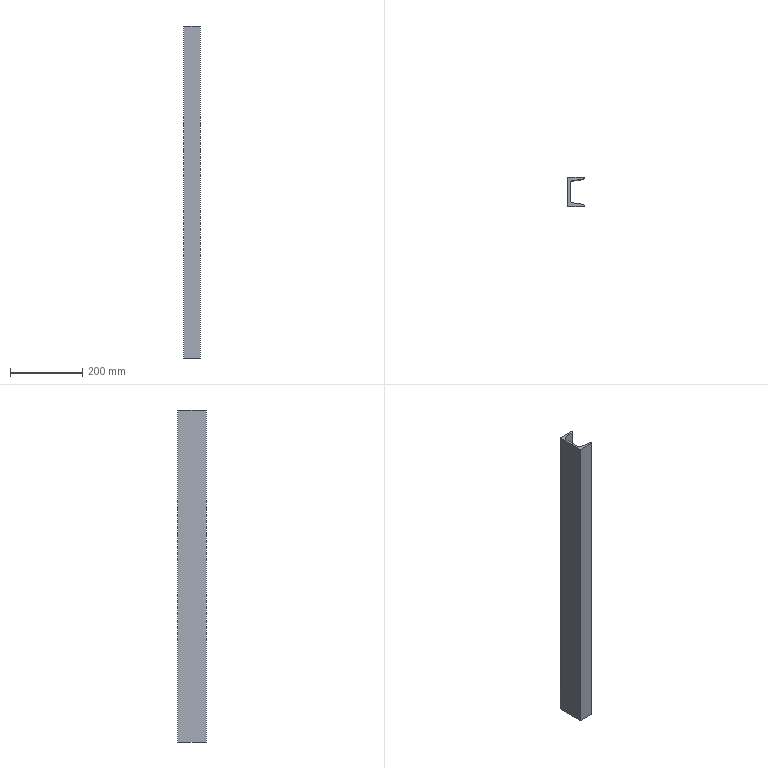Part | SolidWorks | features Extrusion 1 | 1 solid | 14 faces | box 45 x 80 x 920 mm | volume 998999 mm3 | plane 10 | cylinder 4 | commonest cylinder face diameters 8 x2 16 x2
STEP:
#1=CARTESIAN_POINT('',(-3.443,-5.322,0.));
#2=VERTEX_POINT('',#1);
#3=CARTESIAN_POINT('',(0.,-1.361,0.));
#4=VERTEX_POINT('',#3);
#5=CARTESIAN_POINT('',(-4.,-1.361,0.));
#6=DIRECTION('',(0.,0.,1.));
#7=DIRECTION('',(1.,0.,0.));
#8=AXIS2_PLACEMENT_3D('',#5,#6,#7);
#9=CIRCLE('',#8,4.);
#10=EDGE_CURVE('',#2,#4,#9,.T.);
#11=ORIENTED_EDGE('',*,*,#10,.T.);
#12=CARTESIAN_POINT('',(0.,-1.361,920.));
#13=VERTEX_POINT('',#12);
#14=CARTESIAN_POINT('',(0.,-1.361,920.));
#15=DIRECTION('',(0.,0.,-1.));
#16=VECTOR('',#15,1000.);
#17=LINE('',#14,#16);
#18=EDGE_CURVE('',#13,#4,#17,.T.);
#19=ORIENTED_EDGE('',*,*,#18,.F.);
#20=CARTESIAN_POINT('',(-3.443,-5.322,920.));
#21=VERTEX_POINT('',#20);
#22=CARTESIAN_POINT('',(-4.,-1.361,920.));
#23=DIRECTION('',(0.,0.,1.));
#24=DIRECTION('',(1.,0.,0.));
#25=AXIS2_PLACEMENT_3D('',#22,#23,#24);
#26=CIRCLE('',#25,4.);
#27=EDGE_CURVE('',#21,#13,#26,.T.);
#28=ORIENTED_EDGE('',*,*,#27,.F.);
#29=CARTESIAN_POINT('',(-3.443,-5.322,920.));
#30=DIRECTION('',(0.,0.,-1.));
#31=VECTOR('',#30,1000.);
#32=LINE('',#29,#31);
#33=EDGE_CURVE('',#21,#2,#32,.T.);
#34=ORIENTED_EDGE('',*,*,#33,.T.);
#35=EDGE_LOOP('',(#11,#19,#28,#34));
#36=FACE_OUTER_BOUND('',#35,.T.);
#37=CARTESIAN_POINT('',(-4.,-1.361,920.));
#38=DIRECTION('',(0.,0.,-1.));
#39=DIRECTION('',(-1.,0.,0.));
#40=AXIS2_PLACEMENT_3D('',#37,#38,#39);
#41=CYLINDRICAL_SURFACE('',#40,4.);
#42=ADVANCED_FACE('',(#36),#41,.T.);
#43=CARTESIAN_POINT('',(0.,0.,0.));
#44=VERTEX_POINT('',#43);
#45=CARTESIAN_POINT('',(0.,-1.361,0.));
#46=DIRECTION('',(0.,1.,0.));
#47=VECTOR('',#46,1000.);
#48=LINE('',#45,#47);
#49=EDGE_CURVE('',#4,#44,#48,.T.);
#50=ORIENTED_EDGE('',*,*,#49,.T.);
#51=CARTESIAN_POINT('',(0.,0.,920.));
#52=VERTEX_POINT('',#51);
#53=CARTESIAN_POINT('',(0.,0.,920.));
#54=DIRECTION('',(0.,0.,-1.));
#55=VECTOR('',#54,1000.);
#56=LINE('',#53,#55);
#57=EDGE_CURVE('',#52,#44,#56,.T.);
#58=ORIENTED_EDGE('',*,*,#57,.F.);
#59=CARTESIAN_POINT('',(0.,-1.361,920.));
#60=DIRECTION('',(0.,1.,0.));
#61=VECTOR('',#60,1000.);
#62=LINE('',#59,#61);
#63=EDGE_CURVE('',#13,#52,#62,.T.);
#64=ORIENTED_EDGE('',*,*,#63,.F.);
#65=ORIENTED_EDGE('',*,*,#18,.T.);
#66=EDGE_LOOP('',(#50,#58,#64,#65));
#67=FACE_OUTER_BOUND('',#66,.T.);
#68=CARTESIAN_POINT('',(0.,-1.361,920.));
#69=DIRECTION('',(-1.,0.,0.));
#70=DIRECTION('',(0.,0.,1.));
#71=AXIS2_PLACEMENT_3D('',#68,#69,#70);
#72=PLANE('',#71);
#73=ADVANCED_FACE('',(#67),#72,.F.);
#74=CARTESIAN_POINT('',(-45.,0.,0.));
#75=VERTEX_POINT('',#74);
#76=CARTESIAN_POINT('',(0.,0.,0.));
#77=DIRECTION('',(-1.,0.,0.));
#78=VECTOR('',#77,1000.);
#79=LINE('',#76,#78);
#80=EDGE_CURVE('',#44,#75,#79,.T.);
#81=ORIENTED_EDGE('',*,*,#80,.T.);
#82=CARTESIAN_POINT('',(-45.,0.,920.));
#83=VERTEX_POINT('',#82);
#84=CARTESIAN_POINT('',(-45.,0.,920.));
#85=DIRECTION('',(0.,0.,-1.));
#86=VECTOR('',#85,1000.);
#87=LINE('',#84,#86);
#88=EDGE_CURVE('',#83,#75,#87,.T.);
#89=ORIENTED_EDGE('',*,*,#88,.F.);
#90=CARTESIAN_POINT('',(0.,0.,920.));
#91=DIRECTION('',(-1.,0.,0.));
#92=VECTOR('',#91,1000.);
#93=LINE('',#90,#92);
#94=EDGE_CURVE('',#52,#83,#93,.T.);
#95=ORIENTED_EDGE('',*,*,#94,.F.);
#96=ORIENTED_EDGE('',*,*,#57,.T.);
#97=EDGE_LOOP('',(#81,#89,#95,#96));
#98=FACE_OUTER_BOUND('',#97,.T.);
#99=CARTESIAN_POINT('',(0.,0.,920.));
#100=DIRECTION('',(0.,-1.,0.));
#101=DIRECTION('',(1.,0.,0.));
#102=AXIS2_PLACEMENT_3D('',#99,#100,#101);
#103=PLANE('',#102);
#104=ADVANCED_FACE('',(#98),#103,.F.);
#105=CARTESIAN_POINT('',(-45.,-80.,0.));
#106=VERTEX_POINT('',#105);
#107=CARTESIAN_POINT('',(-45.,0.,0.));
#108=DIRECTION('',(0.,-1.,0.));
#109=VECTOR('',#108,1000.);
#110=LINE('',#107,#109);
#111=EDGE_CURVE('',#75,#106,#110,.T.);
#112=ORIENTED_EDGE('',*,*,#111,.T.);
#113=CARTESIAN_POINT('',(-45.,-80.,920.));
#114=VERTEX_POINT('',#113);
#115=CARTESIAN_POINT('',(-45.,-80.,920.));
#116=DIRECTION('',(0.,0.,-1.));
#117=VECTOR('',#116,1000.);
#118=LINE('',#115,#117);
#119=EDGE_CURVE('',#114,#106,#118,.T.);
#120=ORIENTED_EDGE('',*,*,#119,.F.);
#121=CARTESIAN_POINT('',(-45.,0.,920.));
#122=DIRECTION('',(0.,-1.,0.));
#123=VECTOR('',#122,1000.);
#124=LINE('',#121,#123);
#125=EDGE_CURVE('',#83,#114,#124,.T.);
#126=ORIENTED_EDGE('',*,*,#125,.F.);
#127=ORIENTED_EDGE('',*,*,#88,.T.);
#128=EDGE_LOOP('',(#112,#120,#126,#127));
#129=FACE_OUTER_BOUND('',#128,.T.);
#130=CARTESIAN_POINT('',(-45.,0.,920.));
#131=DIRECTION('',(1.,0.,0.));
#132=DIRECTION('',(0.,1.,0.));
#133=AXIS2_PLACEMENT_3D('',#130,#131,#132);
#134=PLANE('',#133);
#135=ADVANCED_FACE('',(#129),#134,.F.);
#136=CARTESIAN_POINT('',(0.,-80.,0.));
#137=VERTEX_POINT('',#136);
#138=CARTESIAN_POINT('',(-45.,-80.,0.));
#139=DIRECTION('',(1.,0.,0.));
#140=VECTOR('',#139,1000.);
#141=LINE('',#138,#140);
#142=EDGE_CURVE('',#106,#137,#141,.T.);
#143=ORIENTED_EDGE('',*,*,#142,.T.);
#144=CARTESIAN_POINT('',(0.,-80.,920.));
#145=VERTEX_POINT('',#144);
#146=CARTESIAN_POINT('',(0.,-80.,920.));
#147=DIRECTION('',(0.,0.,-1.));
#148=VECTOR('',#147,1000.);
#149=LINE('',#146,#148);
#150=EDGE_CURVE('',#145,#137,#149,.T.);
#151=ORIENTED_EDGE('',*,*,#150,.F.);
#152=CARTESIAN_POINT('',(-45.,-80.,920.));
#153=DIRECTION('',(1.,0.,0.));
#154=VECTOR('',#153,1000.);
#155=LINE('',#152,#154);
#156=EDGE_CURVE('',#114,#145,#155,.T.);
#157=ORIENTED_EDGE('',*,*,#156,.F.);
#158=ORIENTED_EDGE('',*,*,#119,.T.);
#159=EDGE_LOOP('',(#143,#151,#157,#158));
#160=FACE_OUTER_BOUND('',#159,.T.);
#161=CARTESIAN_POINT('',(-45.,-80.,920.));
#162=DIRECTION('',(0.,1.,0.));
#163=DIRECTION('',(-1.,0.,0.));
#164=AXIS2_PLACEMENT_3D('',#161,#162,#163);
#165=PLANE('',#164);
#166=ADVANCED_FACE('',(#160),#165,.F.);
#167=CARTESIAN_POINT('',(0.,-78.639,0.));
#168=VERTEX_POINT('',#167);
#169=CARTESIAN_POINT('',(0.,-80.,0.));
#170=DIRECTION('',(0.,1.,0.));
#171=VECTOR('',#170,1000.);
#172=LINE('',#169,#171);
#173=EDGE_CURVE('',#137,#168,#172,.T.);
#174=ORIENTED_EDGE('',*,*,#173,.T.);
#175=CARTESIAN_POINT('',(0.,-78.639,920.));
#176=VERTEX_POINT('',#175);
#177=CARTESIAN_POINT('',(0.,-78.639,920.));
#178=DIRECTION('',(0.,0.,-1.));
#179=VECTOR('',#178,1000.);
#180=LINE('',#177,#179);
#181=EDGE_CURVE('',#176,#168,#180,.T.);
#182=ORIENTED_EDGE('',*,*,#181,.F.);
#183=CARTESIAN_POINT('',(0.,-80.,920.));
#184=DIRECTION('',(0.,1.,0.));
#185=VECTOR('',#184,1000.);
#186=LINE('',#183,#185);
#187=EDGE_CURVE('',#145,#176,#186,.T.);
#188=ORIENTED_EDGE('',*,*,#187,.F.);
#189=ORIENTED_EDGE('',*,*,#150,.T.);
#190=EDGE_LOOP('',(#174,#182,#188,#189));
#191=FACE_OUTER_BOUND('',#190,.T.);
#192=CARTESIAN_POINT('',(0.,-80.,920.));
#193=DIRECTION('',(-1.,0.,0.));
#194=DIRECTION('',(0.,0.,1.));
#195=AXIS2_PLACEMENT_3D('',#192,#193,#194);
#196=PLANE('',#195);
#197=ADVANCED_FACE('',(#191),#196,.F.);
#198=CARTESIAN_POINT('',(-3.443,-74.678,0.));
#199=VERTEX_POINT('',#198);
#200=CARTESIAN_POINT('',(-4.,-78.639,0.));
#201=DIRECTION('',(0.,0.,1.));
#202=DIRECTION('',(1.,0.,0.));
#203=AXIS2_PLACEMENT_3D('',#200,#201,#202);
#204=CIRCLE('',#203,4.);
#205=EDGE_CURVE('',#168,#199,#204,.T.);
#206=ORIENTED_EDGE('',*,*,#205,.T.);
#207=CARTESIAN_POINT('',(-3.443,-74.678,920.));
#208=VERTEX_POINT('',#207);
#209=CARTESIAN_POINT('',(-3.443,-74.678,920.));
#210=DIRECTION('',(0.,0.,-1.));
#211=VECTOR('',#210,1000.);
#212=LINE('',#209,#211);
#213=EDGE_CURVE('',#208,#199,#212,.T.);
#214=ORIENTED_EDGE('',*,*,#213,.F.);
#215=CARTESIAN_POINT('',(-4.,-78.639,920.));
#216=DIRECTION('',(0.,0.,1.));
#217=DIRECTION('',(1.,0.,0.));
#218=AXIS2_PLACEMENT_3D('',#215,#216,#217);
#219=CIRCLE('',#218,4.);
#220=EDGE_CURVE('',#176,#208,#219,.T.);
#221=ORIENTED_EDGE('',*,*,#220,.F.);
#222=ORIENTED_EDGE('',*,*,#181,.T.);
#223=EDGE_LOOP('',(#206,#214,#221,#222));
#224=FACE_OUTER_BOUND('',#223,.T.);
#225=CARTESIAN_POINT('',(-4.,-78.639,920.));
#226=DIRECTION('',(0.,0.,-1.));
#227=DIRECTION('',(-1.,0.,0.));
#228=AXIS2_PLACEMENT_3D('',#225,#226,#227);
#229=CYLINDRICAL_SURFACE('',#228,4.);
#230=ADVANCED_FACE('',(#224),#229,.T.);
#231=CARTESIAN_POINT('',(-32.113,-70.649,0.));
#232=VERTEX_POINT('',#231);
#233=CARTESIAN_POINT('',(-3.443,-74.678,0.));
#234=DIRECTION('',(-0.9903,0.1392,0.));
#235=VECTOR('',#234,1000.);
#236=LINE('',#233,#235);
#237=EDGE_CURVE('',#199,#232,#236,.T.);
#238=ORIENTED_EDGE('',*,*,#237,.T.);
#239=CARTESIAN_POINT('',(-32.113,-70.649,920.));
#240=VERTEX_POINT('',#239);
#241=CARTESIAN_POINT('',(-32.113,-70.649,920.));
#242=DIRECTION('',(0.,0.,-1.));
#243=VECTOR('',#242,1000.);
#244=LINE('',#241,#243);
#245=EDGE_CURVE('',#240,#232,#244,.T.);
#246=ORIENTED_EDGE('',*,*,#245,.F.);
#247=CARTESIAN_POINT('',(-3.443,-74.678,920.));
#248=DIRECTION('',(-0.9903,0.1392,0.));
#249=VECTOR('',#248,1000.);
#250=LINE('',#247,#249);
#251=EDGE_CURVE('',#208,#240,#250,.T.);
#252=ORIENTED_EDGE('',*,*,#251,.F.);
#253=ORIENTED_EDGE('',*,*,#213,.T.);
#254=EDGE_LOOP('',(#238,#246,#252,#253));
#255=FACE_OUTER_BOUND('',#254,.T.);
#256=CARTESIAN_POINT('',(-3.443,-74.678,920.));
#257=DIRECTION('',(-0.1392,-0.9903,0.));
#258=DIRECTION('',(0.9903,-0.1392,0.));
#259=AXIS2_PLACEMENT_3D('',#256,#257,#258);
#260=PLANE('',#259);
#261=ADVANCED_FACE('',(#255),#260,.F.);
#262=CARTESIAN_POINT('',(-39.,-62.727,0.));
#263=VERTEX_POINT('',#262);
#264=CARTESIAN_POINT('',(-31.,-62.727,0.));
#265=DIRECTION('',(0.,0.,-1.));
#266=DIRECTION('',(-1.,0.,0.));
#267=AXIS2_PLACEMENT_3D('',#264,#265,#266);
#268=CIRCLE('',#267,8.);
#269=EDGE_CURVE('',#232,#263,#268,.T.);
#270=ORIENTED_EDGE('',*,*,#269,.T.);
#271=CARTESIAN_POINT('',(-39.,-62.727,920.));
#272=VERTEX_POINT('',#271);
#273=CARTESIAN_POINT('',(-39.,-62.727,920.));
#274=DIRECTION('',(0.,0.,-1.));
#275=VECTOR('',#274,1000.);
#276=LINE('',#273,#275);
#277=EDGE_CURVE('',#272,#263,#276,.T.);
#278=ORIENTED_EDGE('',*,*,#277,.F.);
#279=CARTESIAN_POINT('',(-31.,-62.727,920.));
#280=DIRECTION('',(0.,0.,-1.));
#281=DIRECTION('',(-1.,0.,0.));
#282=AXIS2_PLACEMENT_3D('',#279,#280,#281);
#283=CIRCLE('',#282,8.);
#284=EDGE_CURVE('',#240,#272,#283,.T.);
#285=ORIENTED_EDGE('',*,*,#284,.F.);
#286=ORIENTED_EDGE('',*,*,#245,.T.);
#287=EDGE_LOOP('',(#270,#278,#285,#286));
#288=FACE_OUTER_BOUND('',#287,.T.);
#289=CARTESIAN_POINT('',(-31.,-62.727,920.));
#290=DIRECTION('',(0.,0.,-1.));
#291=DIRECTION('',(-1.,0.,0.));
#292=AXIS2_PLACEMENT_3D('',#289,#290,#291);
#293=CYLINDRICAL_SURFACE('',#292,8.);
#294=ADVANCED_FACE('',(#288),#293,.F.);
#295=CARTESIAN_POINT('',(-39.,-17.273,0.));
#296=VERTEX_POINT('',#295);
#297=CARTESIAN_POINT('',(-39.,-62.727,0.));
#298=DIRECTION('',(0.,1.,0.));
#299=VECTOR('',#298,1000.);
#300=LINE('',#297,#299);
#301=EDGE_CURVE('',#263,#296,#300,.T.);
#302=ORIENTED_EDGE('',*,*,#301,.T.);
#303=CARTESIAN_POINT('',(-39.,-17.273,920.));
#304=VERTEX_POINT('',#303);
#305=CARTESIAN_POINT('',(-39.,-17.273,920.));
#306=DIRECTION('',(0.,0.,-1.));
#307=VECTOR('',#306,1000.);
#308=LINE('',#305,#307);
#309=EDGE_CURVE('',#304,#296,#308,.T.);
#310=ORIENTED_EDGE('',*,*,#309,.F.);
#311=CARTESIAN_POINT('',(-39.,-62.727,920.));
#312=DIRECTION('',(0.,1.,0.));
#313=VECTOR('',#312,1000.);
#314=LINE('',#311,#313);
#315=EDGE_CURVE('',#272,#304,#314,.T.);
#316=ORIENTED_EDGE('',*,*,#315,.F.);
#317=ORIENTED_EDGE('',*,*,#277,.T.);
#318=EDGE_LOOP('',(#302,#310,#316,#317));
#319=FACE_OUTER_BOUND('',#318,.T.);
#320=CARTESIAN_POINT('',(-39.,-62.727,920.));
#321=DIRECTION('',(-1.,0.,0.));
#322=DIRECTION('',(0.,0.,1.));
#323=AXIS2_PLACEMENT_3D('',#320,#321,#322);
#324=PLANE('',#323);
#325=ADVANCED_FACE('',(#319),#324,.F.);
#326=CARTESIAN_POINT('',(-32.113,-9.351,0.));
#327=VERTEX_POINT('',#326);
#328=CARTESIAN_POINT('',(-31.,-17.273,0.));
#329=DIRECTION('',(0.,0.,-1.));
#330=DIRECTION('',(-1.,0.,0.));
#331=AXIS2_PLACEMENT_3D('',#328,#329,#330);
#332=CIRCLE('',#331,8.);
#333=EDGE_CURVE('',#296,#327,#332,.T.);
#334=ORIENTED_EDGE('',*,*,#333,.T.);
#335=CARTESIAN_POINT('',(-32.113,-9.351,920.));
#336=VERTEX_POINT('',#335);
#337=CARTESIAN_POINT('',(-32.113,-9.351,920.));
#338=DIRECTION('',(0.,0.,-1.));
#339=VECTOR('',#338,1000.);
#340=LINE('',#337,#339);
#341=EDGE_CURVE('',#336,#327,#340,.T.);
#342=ORIENTED_EDGE('',*,*,#341,.F.);
#343=CARTESIAN_POINT('',(-31.,-17.273,920.));
#344=DIRECTION('',(0.,0.,-1.));
#345=DIRECTION('',(-1.,0.,0.));
#346=AXIS2_PLACEMENT_3D('',#343,#344,#345);
#347=CIRCLE('',#346,8.);
#348=EDGE_CURVE('',#304,#336,#347,.T.);
#349=ORIENTED_EDGE('',*,*,#348,.F.);
#350=ORIENTED_EDGE('',*,*,#309,.T.);
#351=EDGE_LOOP('',(#334,#342,#349,#350));
#352=FACE_OUTER_BOUND('',#351,.T.);
#353=CARTESIAN_POINT('',(-31.,-17.273,920.));
#354=DIRECTION('',(0.,0.,-1.));
#355=DIRECTION('',(-1.,0.,0.));
#356=AXIS2_PLACEMENT_3D('',#353,#354,#355);
#357=CYLINDRICAL_SURFACE('',#356,8.);
#358=ADVANCED_FACE('',(#352),#357,.F.);
#359=CARTESIAN_POINT('',(-32.113,-9.351,0.));
#360=DIRECTION('',(0.9903,0.1392,0.));
#361=VECTOR('',#360,1000.);
#362=LINE('',#359,#361);
#363=EDGE_CURVE('',#327,#2,#362,.T.);
#364=ORIENTED_EDGE('',*,*,#363,.T.);
#365=ORIENTED_EDGE('',*,*,#33,.F.);
#366=CARTESIAN_POINT('',(-32.113,-9.351,920.));
#367=DIRECTION('',(0.9903,0.1392,0.));
#368=VECTOR('',#367,1000.);
#369=LINE('',#366,#368);
#370=EDGE_CURVE('',#336,#21,#369,.T.);
#371=ORIENTED_EDGE('',*,*,#370,.F.);
#372=ORIENTED_EDGE('',*,*,#341,.T.);
#373=EDGE_LOOP('',(#364,#365,#371,#372));
#374=FACE_OUTER_BOUND('',#373,.T.);
#375=CARTESIAN_POINT('',(-32.113,-9.351,920.));
#376=DIRECTION('',(-0.1392,0.9903,0.));
#377=DIRECTION('',(-0.9903,-0.1392,0.));
#378=AXIS2_PLACEMENT_3D('',#375,#376,#377);
#379=PLANE('',#378);
#380=ADVANCED_FACE('',(#374),#379,.F.);
#381=ORIENTED_EDGE('',*,*,#27,.T.);
#382=ORIENTED_EDGE('',*,*,#63,.T.);
#383=ORIENTED_EDGE('',*,*,#94,.T.);
#384=ORIENTED_EDGE('',*,*,#125,.T.);
#385=ORIENTED_EDGE('',*,*,#156,.T.);
#386=ORIENTED_EDGE('',*,*,#187,.T.);
#387=ORIENTED_EDGE('',*,*,#220,.T.);
#388=ORIENTED_EDGE('',*,*,#251,.T.);
#389=ORIENTED_EDGE('',*,*,#284,.T.);
#390=ORIENTED_EDGE('',*,*,#315,.T.);
#391=ORIENTED_EDGE('',*,*,#348,.T.);
#392=ORIENTED_EDGE('',*,*,#370,.T.);
#393=EDGE_LOOP('',(#381,#382,#383,#384,#385,#386,#387,#388,#389,#390,#391,#392));
#394=FACE_OUTER_BOUND('',#393,.T.);
#395=CARTESIAN_POINT('',(-4.,-1.361,920.));
#396=DIRECTION('',(0.,0.,1.));
#397=DIRECTION('',(1.,0.,0.));
#398=AXIS2_PLACEMENT_3D('',#395,#396,#397);
#399=PLANE('',#398);
#400=ADVANCED_FACE('',(#394),#399,.T.);
#401=ORIENTED_EDGE('',*,*,#10,.F.);
#402=ORIENTED_EDGE('',*,*,#363,.F.);
#403=ORIENTED_EDGE('',*,*,#333,.F.);
#404=ORIENTED_EDGE('',*,*,#301,.F.);
#405=ORIENTED_EDGE('',*,*,#269,.F.);
#406=ORIENTED_EDGE('',*,*,#237,.F.);
#407=ORIENTED_EDGE('',*,*,#205,.F.);
#408=ORIENTED_EDGE('',*,*,#173,.F.);
#409=ORIENTED_EDGE('',*,*,#142,.F.);
#410=ORIENTED_EDGE('',*,*,#111,.F.);
#411=ORIENTED_EDGE('',*,*,#80,.F.);
#412=ORIENTED_EDGE('',*,*,#49,.F.);
#413=EDGE_LOOP('',(#401,#402,#403,#404,#405,#406,#407,#408,#409,#410,#411,#412));
#414=FACE_OUTER_BOUND('',#413,.T.);
#415=CARTESIAN_POINT('',(-4.,-1.361,0.));
#416=DIRECTION('',(0.,0.,1.));
#417=DIRECTION('',(1.,0.,0.));
#418=AXIS2_PLACEMENT_3D('',#415,#416,#417);
#419=PLANE('',#418);
#420=ADVANCED_FACE('',(#414),#419,.F.);
#421=CLOSED_SHELL('',(#42,#73,#104,#135,#166,#197,#230,#261,#294,#325,#358,#380,#400,#420));
#422=MANIFOLD_SOLID_BREP('',#421);
#423=CARTESIAN_POINT('',(0.,0.,0.));
#424=DIRECTION('',(0.,0.,1.));
#425=DIRECTION('',(1.,0.,0.));
#426=AXIS2_PLACEMENT_3D('',#423,#424,#425);
#427=(LENGTH_UNIT()NAMED_UNIT(*)SI_UNIT(.MILLI.,.METRE.));
#428=UNCERTAINTY_MEASURE_WITH_UNIT(LENGTH_MEASURE(0.00001),#427,'','');
#429=(NAMED_UNIT(*)PLANE_ANGLE_UNIT()SI_UNIT($,.RADIAN.));
#430=(NAMED_UNIT(*)SI_UNIT($,.STERADIAN.)SOLID_ANGLE_UNIT());
#431=(GEOMETRIC_REPRESENTATION_CONTEXT(3)GLOBAL_UNCERTAINTY_ASSIGNED_CONTEXT((#428))GLOBAL_UNIT_ASSIGNED_CONTEXT((#427,#429,#430))REPRESENTATION_CONTEXT('',''));
#432=ADVANCED_BREP_SHAPE_REPRESENTATION('',(#422,#426),#431);